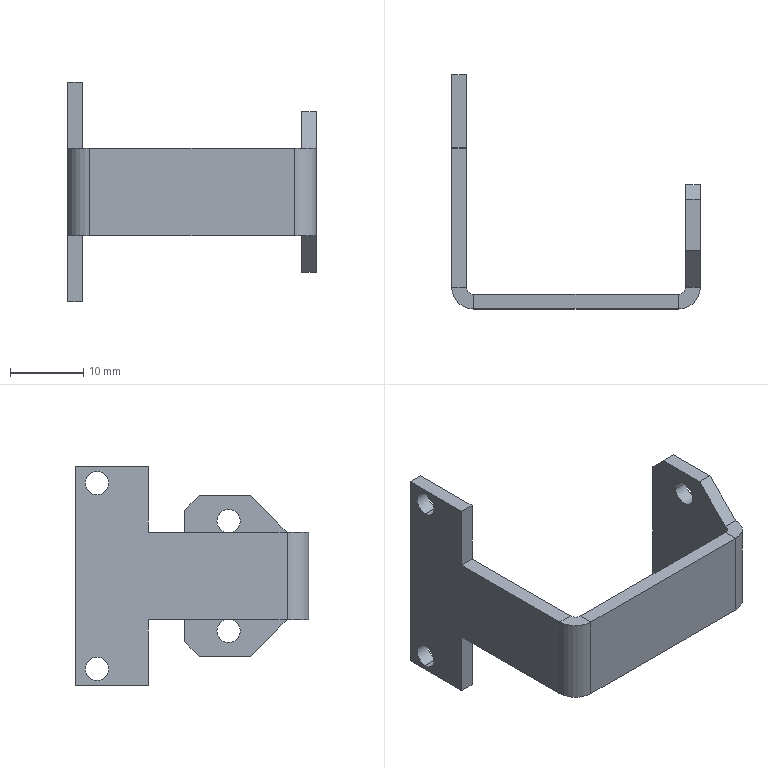Part | SolidWorks | features ICE 5, Chamfer 1, FlatPattern 1, SMBaseFlange 1, SheetMetal 1 | 1 solid | 38 faces | box 34 x 32 x 30 mm | volume 2372 mm3 | plane 26 | cylinder 12 | commonest cylinder face diameters 3.2 x8 2 x2 6 x2
STEP:
#1=CARTESIAN_POINT('',(-30.,12.,26.1));
#2=VERTEX_POINT('',#1);
#3=CARTESIAN_POINT('',(-30.,12.,29.3));
#4=VERTEX_POINT('',#3);
#5=CARTESIAN_POINT('',(-30.,12.,27.7));
#6=DIRECTION('',(-1.,0.,0.));
#7=DIRECTION('',(0.,-1.,0.));
#8=AXIS2_PLACEMENT_3D('',#5,#6,#7);
#9=CIRCLE('',#8,1.6);
#10=EDGE_CURVE('',#2,#4,#9,.T.);
#11=ORIENTED_EDGE('',*,*,#10,.F.);
#12=CARTESIAN_POINT('',(-32.,12.,26.1));
#13=VERTEX_POINT('',#12);
#14=CARTESIAN_POINT('',(-27.,12.,26.1));
#15=DIRECTION('',(-1.,0.,0.));
#16=VECTOR('',#15,1000.);
#17=LINE('',#14,#16);
#18=EDGE_CURVE('',#2,#13,#17,.T.);
#19=ORIENTED_EDGE('',*,*,#18,.T.);
#20=CARTESIAN_POINT('',(-32.,12.,29.3));
#21=VERTEX_POINT('',#20);
#22=CARTESIAN_POINT('',(-32.,12.,27.7));
#23=DIRECTION('',(-1.,0.,0.));
#24=DIRECTION('',(0.,0.,1.));
#25=AXIS2_PLACEMENT_3D('',#22,#23,#24);
#26=CIRCLE('',#25,1.6);
#27=EDGE_CURVE('',#13,#21,#26,.T.);
#28=ORIENTED_EDGE('',*,*,#27,.T.);
#29=CARTESIAN_POINT('',(-27.,12.,29.3));
#30=DIRECTION('',(-1.,0.,0.));
#31=VECTOR('',#30,1000.);
#32=LINE('',#29,#31);
#33=EDGE_CURVE('',#4,#21,#32,.T.);
#34=ORIENTED_EDGE('',*,*,#33,.F.);
#35=EDGE_LOOP('',(#11,#19,#28,#34));
#36=FACE_OUTER_BOUND('',#35,.T.);
#37=CARTESIAN_POINT('',(-27.,12.,27.7));
#38=DIRECTION('',(-1.,0.,0.));
#39=DIRECTION('',(0.,0.,1.));
#40=AXIS2_PLACEMENT_3D('',#37,#38,#39);
#41=CYLINDRICAL_SURFACE('',#40,1.6);
#42=ADVANCED_FACE('',(#36),#41,.F.);
#43=CARTESIAN_POINT('',(-30.,12.,0.7));
#44=VERTEX_POINT('',#43);
#45=CARTESIAN_POINT('',(-30.,12.,3.9));
#46=VERTEX_POINT('',#45);
#47=CARTESIAN_POINT('',(-30.,12.,2.3));
#48=DIRECTION('',(-1.,0.,0.));
#49=DIRECTION('',(0.,-1.,0.));
#50=AXIS2_PLACEMENT_3D('',#47,#48,#49);
#51=CIRCLE('',#50,1.6);
#52=EDGE_CURVE('',#44,#46,#51,.T.);
#53=ORIENTED_EDGE('',*,*,#52,.F.);
#54=CARTESIAN_POINT('',(-32.,12.,0.7));
#55=VERTEX_POINT('',#54);
#56=CARTESIAN_POINT('',(-27.,12.,0.7));
#57=DIRECTION('',(-1.,0.,0.));
#58=VECTOR('',#57,1000.);
#59=LINE('',#56,#58);
#60=EDGE_CURVE('',#44,#55,#59,.T.);
#61=ORIENTED_EDGE('',*,*,#60,.T.);
#62=CARTESIAN_POINT('',(-32.,12.,3.9));
#63=VERTEX_POINT('',#62);
#64=CARTESIAN_POINT('',(-32.,12.,2.3));
#65=DIRECTION('',(-1.,0.,0.));
#66=DIRECTION('',(0.,0.,1.));
#67=AXIS2_PLACEMENT_3D('',#64,#65,#66);
#68=CIRCLE('',#67,1.6);
#69=EDGE_CURVE('',#55,#63,#68,.T.);
#70=ORIENTED_EDGE('',*,*,#69,.T.);
#71=CARTESIAN_POINT('',(-27.,12.,3.9));
#72=DIRECTION('',(-1.,0.,0.));
#73=VECTOR('',#72,1000.);
#74=LINE('',#71,#73);
#75=EDGE_CURVE('',#46,#63,#74,.T.);
#76=ORIENTED_EDGE('',*,*,#75,.F.);
#77=EDGE_LOOP('',(#53,#61,#70,#76));
#78=FACE_OUTER_BOUND('',#77,.T.);
#79=CARTESIAN_POINT('',(-27.,12.,2.3));
#80=DIRECTION('',(-1.,0.,0.));
#81=DIRECTION('',(0.,0.,1.));
#82=AXIS2_PLACEMENT_3D('',#79,#80,#81);
#83=CYLINDRICAL_SURFACE('',#82,1.6);
#84=ADVANCED_FACE('',(#78),#83,.F.);
#85=CARTESIAN_POINT('',(0.,-7.6,7.5));
#86=VERTEX_POINT('',#85);
#87=CARTESIAN_POINT('',(0.,-4.4,7.5));
#88=VERTEX_POINT('',#87);
#89=CARTESIAN_POINT('',(0.,-6.,7.5));
#90=DIRECTION('',(1.,0.,0.));
#91=DIRECTION('',(0.,1.,0.));
#92=AXIS2_PLACEMENT_3D('',#89,#90,#91);
#93=CIRCLE('',#92,1.6);
#94=EDGE_CURVE('',#86,#88,#93,.T.);
#95=ORIENTED_EDGE('',*,*,#94,.F.);
#96=CARTESIAN_POINT('',(2.,-7.6,7.5));
#97=VERTEX_POINT('',#96);
#98=CARTESIAN_POINT('',(-8.,-7.6,7.5));
#99=DIRECTION('',(1.,0.,0.));
#100=VECTOR('',#99,1000.);
#101=LINE('',#98,#100);
#102=EDGE_CURVE('',#86,#97,#101,.T.);
#103=ORIENTED_EDGE('',*,*,#102,.T.);
#104=CARTESIAN_POINT('',(2.,-4.4,7.5));
#105=VERTEX_POINT('',#104);
#106=CARTESIAN_POINT('',(2.,-6.,7.5));
#107=DIRECTION('',(1.,0.,0.));
#108=DIRECTION('',(0.,1.,0.));
#109=AXIS2_PLACEMENT_3D('',#106,#107,#108);
#110=CIRCLE('',#109,1.6);
#111=EDGE_CURVE('',#97,#105,#110,.T.);
#112=ORIENTED_EDGE('',*,*,#111,.T.);
#113=CARTESIAN_POINT('',(-8.,-4.4,7.5));
#114=DIRECTION('',(1.,0.,0.));
#115=VECTOR('',#114,1000.);
#116=LINE('',#113,#115);
#117=EDGE_CURVE('',#88,#105,#116,.T.);
#118=ORIENTED_EDGE('',*,*,#117,.F.);
#119=EDGE_LOOP('',(#95,#103,#112,#118));
#120=FACE_OUTER_BOUND('',#119,.T.);
#121=CARTESIAN_POINT('',(-8.,-6.,7.5));
#122=DIRECTION('',(1.,0.,0.));
#123=DIRECTION('',(0.,1.,0.));
#124=AXIS2_PLACEMENT_3D('',#121,#122,#123);
#125=CYLINDRICAL_SURFACE('',#124,1.6);
#126=ADVANCED_FACE('',(#120),#125,.F.);
#127=CARTESIAN_POINT('',(0.,-7.6,22.5));
#128=VERTEX_POINT('',#127);
#129=CARTESIAN_POINT('',(0.,-4.4,22.5));
#130=VERTEX_POINT('',#129);
#131=CARTESIAN_POINT('',(0.,-6.,22.5));
#132=DIRECTION('',(1.,0.,0.));
#133=DIRECTION('',(0.,1.,0.));
#134=AXIS2_PLACEMENT_3D('',#131,#132,#133);
#135=CIRCLE('',#134,1.6);
#136=EDGE_CURVE('',#128,#130,#135,.T.);
#137=ORIENTED_EDGE('',*,*,#136,.F.);
#138=CARTESIAN_POINT('',(2.,-7.6,22.5));
#139=VERTEX_POINT('',#138);
#140=CARTESIAN_POINT('',(-8.,-7.6,22.5));
#141=DIRECTION('',(1.,0.,0.));
#142=VECTOR('',#141,1000.);
#143=LINE('',#140,#142);
#144=EDGE_CURVE('',#128,#139,#143,.T.);
#145=ORIENTED_EDGE('',*,*,#144,.T.);
#146=CARTESIAN_POINT('',(2.,-4.4,22.5));
#147=VERTEX_POINT('',#146);
#148=CARTESIAN_POINT('',(2.,-6.,22.5));
#149=DIRECTION('',(1.,0.,0.));
#150=DIRECTION('',(0.,1.,0.));
#151=AXIS2_PLACEMENT_3D('',#148,#149,#150);
#152=CIRCLE('',#151,1.6);
#153=EDGE_CURVE('',#139,#147,#152,.T.);
#154=ORIENTED_EDGE('',*,*,#153,.T.);
#155=CARTESIAN_POINT('',(-8.,-4.4,22.5));
#156=DIRECTION('',(1.,0.,0.));
#157=VECTOR('',#156,1000.);
#158=LINE('',#155,#157);
#159=EDGE_CURVE('',#130,#147,#158,.T.);
#160=ORIENTED_EDGE('',*,*,#159,.F.);
#161=EDGE_LOOP('',(#137,#145,#154,#160));
#162=FACE_OUTER_BOUND('',#161,.T.);
#163=CARTESIAN_POINT('',(-8.,-6.,22.5));
#164=DIRECTION('',(1.,0.,0.));
#165=DIRECTION('',(0.,1.,0.));
#166=AXIS2_PLACEMENT_3D('',#163,#164,#165);
#167=CYLINDRICAL_SURFACE('',#166,1.6);
#168=ADVANCED_FACE('',(#162),#167,.F.);
#169=CARTESIAN_POINT('',(2.,-6.,7.5));
#170=DIRECTION('',(1.,0.,0.));
#171=DIRECTION('',(0.,1.,0.));
#172=AXIS2_PLACEMENT_3D('',#169,#170,#171);
#173=CIRCLE('',#172,1.6);
#174=EDGE_CURVE('',#105,#97,#173,.T.);
#175=ORIENTED_EDGE('',*,*,#174,.F.);
#176=ORIENTED_EDGE('',*,*,#111,.F.);
#177=EDGE_LOOP('',(#175,#176));
#178=FACE_BOUND('',#177,.T.);
#179=CARTESIAN_POINT('',(2.,-6.,22.5));
#180=DIRECTION('',(1.,0.,0.));
#181=DIRECTION('',(0.,1.,0.));
#182=AXIS2_PLACEMENT_3D('',#179,#180,#181);
#183=CIRCLE('',#182,1.6);
#184=EDGE_CURVE('',#147,#139,#183,.T.);
#185=ORIENTED_EDGE('',*,*,#184,.F.);
#186=ORIENTED_EDGE('',*,*,#153,.F.);
#187=EDGE_LOOP('',(#185,#186));
#188=FACE_BOUND('',#187,.T.);
#189=CARTESIAN_POINT('',(2.,0.,24.));
#190=VERTEX_POINT('',#189);
#191=CARTESIAN_POINT('',(2.,0.,6.));
#192=VERTEX_POINT('',#191);
#193=CARTESIAN_POINT('',(2.,0.,30.));
#194=DIRECTION('',(0.,0.,-1.));
#195=VECTOR('',#194,1000.);
#196=LINE('',#193,#195);
#197=EDGE_CURVE('',#190,#192,#196,.T.);
#198=ORIENTED_EDGE('',*,*,#197,.F.);
#199=CARTESIAN_POINT('',(2.,-2.,26.));
#200=VERTEX_POINT('',#199);
#201=CARTESIAN_POINT('',(2.,-3.,27.));
#202=DIRECTION('',(0.,-0.7071,0.7071));
#203=VECTOR('',#202,1000.);
#204=LINE('',#201,#203);
#205=EDGE_CURVE('',#190,#200,#204,.T.);
#206=ORIENTED_EDGE('',*,*,#205,.T.);
#207=CARTESIAN_POINT('',(2.,-9.,26.));
#208=VERTEX_POINT('',#207);
#209=CARTESIAN_POINT('',(2.,0.,26.));
#210=DIRECTION('',(0.,1.,0.));
#211=VECTOR('',#210,1000.);
#212=LINE('',#209,#211);
#213=EDGE_CURVE('',#208,#200,#212,.T.);
#214=ORIENTED_EDGE('',*,*,#213,.F.);
#215=CARTESIAN_POINT('',(2.,-14.,21.));
#216=VERTEX_POINT('',#215);
#217=CARTESIAN_POINT('',(2.,-2.5,32.5));
#218=DIRECTION('',(0.,0.7071,0.7071));
#219=VECTOR('',#218,1000.);
#220=LINE('',#217,#219);
#221=EDGE_CURVE('',#216,#208,#220,.T.);
#222=ORIENTED_EDGE('',*,*,#221,.F.);
#223=CARTESIAN_POINT('',(2.,-14.,9.));
#224=VERTEX_POINT('',#223);
#225=CARTESIAN_POINT('',(2.,-14.,30.));
#226=DIRECTION('',(0.,0.,-1.));
#227=VECTOR('',#226,1000.);
#228=LINE('',#225,#227);
#229=EDGE_CURVE('',#216,#224,#228,.T.);
#230=ORIENTED_EDGE('',*,*,#229,.T.);
#231=CARTESIAN_POINT('',(2.,-9.,4.));
#232=VERTEX_POINT('',#231);
#233=CARTESIAN_POINT('',(2.,-17.5,12.5));
#234=DIRECTION('',(0.,-0.7071,0.7071));
#235=VECTOR('',#234,1000.);
#236=LINE('',#233,#235);
#237=EDGE_CURVE('',#232,#224,#236,.T.);
#238=ORIENTED_EDGE('',*,*,#237,.F.);
#239=CARTESIAN_POINT('',(2.,-2.,4.));
#240=VERTEX_POINT('',#239);
#241=CARTESIAN_POINT('',(2.,0.,4.));
#242=DIRECTION('',(0.,-1.,0.));
#243=VECTOR('',#242,1000.);
#244=LINE('',#241,#243);
#245=EDGE_CURVE('',#240,#232,#244,.T.);
#246=ORIENTED_EDGE('',*,*,#245,.F.);
#247=CARTESIAN_POINT('',(2.,12.,18.));
#248=DIRECTION('',(0.,0.7071,0.7071));
#249=VECTOR('',#248,1000.);
#250=LINE('',#247,#249);
#251=EDGE_CURVE('',#240,#192,#250,.T.);
#252=ORIENTED_EDGE('',*,*,#251,.T.);
#253=EDGE_LOOP('',(#198,#206,#214,#222,#230,#238,#246,#252));
#254=FACE_OUTER_BOUND('',#253,.T.);
#255=CARTESIAN_POINT('',(2.,0.,30.));
#256=DIRECTION('',(1.,0.,0.));
#257=DIRECTION('',(0.,1.,0.));
#258=AXIS2_PLACEMENT_3D('',#255,#256,#257);
#259=PLANE('',#258);
#260=ADVANCED_FACE('',(#178,#188,#254),#259,.T.);
#261=CARTESIAN_POINT('',(0.,-6.,7.5));
#262=DIRECTION('',(1.,0.,0.));
#263=DIRECTION('',(0.,1.,0.));
#264=AXIS2_PLACEMENT_3D('',#261,#262,#263);
#265=CIRCLE('',#264,1.6);
#266=EDGE_CURVE('',#88,#86,#265,.T.);
#267=ORIENTED_EDGE('',*,*,#266,.T.);
#268=ORIENTED_EDGE('',*,*,#94,.T.);
#269=EDGE_LOOP('',(#267,#268));
#270=FACE_BOUND('',#269,.T.);
#271=CARTESIAN_POINT('',(0.,-6.,22.5));
#272=DIRECTION('',(1.,0.,0.));
#273=DIRECTION('',(0.,1.,0.));
#274=AXIS2_PLACEMENT_3D('',#271,#272,#273);
#275=CIRCLE('',#274,1.6);
#276=EDGE_CURVE('',#130,#128,#275,.T.);
#277=ORIENTED_EDGE('',*,*,#276,.T.);
#278=ORIENTED_EDGE('',*,*,#136,.T.);
#279=EDGE_LOOP('',(#277,#278));
#280=FACE_BOUND('',#279,.T.);
#281=CARTESIAN_POINT('',(0.,-9.,26.));
#282=VERTEX_POINT('',#281);
#283=CARTESIAN_POINT('',(0.,-2.,26.));
#284=VERTEX_POINT('',#283);
#285=CARTESIAN_POINT('',(0.,0.,26.));
#286=DIRECTION('',(0.,1.,0.));
#287=VECTOR('',#286,1000.);
#288=LINE('',#285,#287);
#289=EDGE_CURVE('',#282,#284,#288,.T.);
#290=ORIENTED_EDGE('',*,*,#289,.T.);
#291=CARTESIAN_POINT('',(0.,0.,24.));
#292=VERTEX_POINT('',#291);
#293=CARTESIAN_POINT('',(0.,0.,24.));
#294=DIRECTION('',(0.,0.7071,-0.7071));
#295=VECTOR('',#294,1000.);
#296=LINE('',#293,#295);
#297=EDGE_CURVE('',#284,#292,#296,.T.);
#298=ORIENTED_EDGE('',*,*,#297,.T.);
#299=CARTESIAN_POINT('',(0.,0.,6.));
#300=VERTEX_POINT('',#299);
#301=CARTESIAN_POINT('',(0.,0.,30.));
#302=DIRECTION('',(0.,0.,-1.));
#303=VECTOR('',#302,1000.);
#304=LINE('',#301,#303);
#305=EDGE_CURVE('',#292,#300,#304,.T.);
#306=ORIENTED_EDGE('',*,*,#305,.T.);
#307=CARTESIAN_POINT('',(0.,-2.,4.));
#308=VERTEX_POINT('',#307);
#309=CARTESIAN_POINT('',(0.,-2.,4.));
#310=DIRECTION('',(0.,-0.7071,-0.7071));
#311=VECTOR('',#310,1000.);
#312=LINE('',#309,#311);
#313=EDGE_CURVE('',#300,#308,#312,.T.);
#314=ORIENTED_EDGE('',*,*,#313,.T.);
#315=CARTESIAN_POINT('',(0.,-9.,4.));
#316=VERTEX_POINT('',#315);
#317=CARTESIAN_POINT('',(0.,0.,4.));
#318=DIRECTION('',(0.,-1.,0.));
#319=VECTOR('',#318,1000.);
#320=LINE('',#317,#319);
#321=EDGE_CURVE('',#308,#316,#320,.T.);
#322=ORIENTED_EDGE('',*,*,#321,.T.);
#323=CARTESIAN_POINT('',(0.,-14.,9.));
#324=VERTEX_POINT('',#323);
#325=CARTESIAN_POINT('',(0.,-17.5,12.5));
#326=DIRECTION('',(0.,-0.7071,0.7071));
#327=VECTOR('',#326,1000.);
#328=LINE('',#325,#327);
#329=EDGE_CURVE('',#316,#324,#328,.T.);
#330=ORIENTED_EDGE('',*,*,#329,.T.);
#331=CARTESIAN_POINT('',(0.,-14.,21.));
#332=VERTEX_POINT('',#331);
#333=CARTESIAN_POINT('',(0.,-14.,30.));
#334=DIRECTION('',(0.,0.,-1.));
#335=VECTOR('',#334,1000.);
#336=LINE('',#333,#335);
#337=EDGE_CURVE('',#332,#324,#336,.T.);
#338=ORIENTED_EDGE('',*,*,#337,.F.);
#339=CARTESIAN_POINT('',(0.,-2.5,32.5));
#340=DIRECTION('',(0.,0.7071,0.7071));
#341=VECTOR('',#340,1000.);
#342=LINE('',#339,#341);
#343=EDGE_CURVE('',#332,#282,#342,.T.);
#344=ORIENTED_EDGE('',*,*,#343,.T.);
#345=EDGE_LOOP('',(#290,#298,#306,#314,#322,#330,#338,#344));
#346=FACE_OUTER_BOUND('',#345,.T.);
#347=CARTESIAN_POINT('',(0.,0.,30.));
#348=DIRECTION('',(1.,0.,0.));
#349=DIRECTION('',(0.,1.,0.));
#350=AXIS2_PLACEMENT_3D('',#347,#348,#349);
#351=PLANE('',#350);
#352=ADVANCED_FACE('',(#270,#280,#346),#351,.F.);
#353=ORIENTED_EDGE('',*,*,#213,.T.);
#354=CARTESIAN_POINT('',(0.,-2.,26.));
#355=DIRECTION('',(-1.,0.,0.));
#356=VECTOR('',#355,1000.);
#357=LINE('',#354,#356);
#358=EDGE_CURVE('',#200,#284,#357,.T.);
#359=ORIENTED_EDGE('',*,*,#358,.T.);
#360=ORIENTED_EDGE('',*,*,#289,.F.);
#361=CARTESIAN_POINT('',(0.,-9.,26.));
#362=DIRECTION('',(1.,0.,0.));
#363=VECTOR('',#362,1000.);
#364=LINE('',#361,#363);
#365=EDGE_CURVE('',#282,#208,#364,.T.);
#366=ORIENTED_EDGE('',*,*,#365,.T.);
#367=EDGE_LOOP('',(#353,#359,#360,#366));
#368=FACE_OUTER_BOUND('',#367,.T.);
#369=CARTESIAN_POINT('',(-8.,0.,26.));
#370=DIRECTION('',(0.,0.,-1.));
#371=DIRECTION('',(0.,1.,0.));
#372=AXIS2_PLACEMENT_3D('',#369,#370,#371);
#373=PLANE('',#372);
#374=ADVANCED_FACE('',(#368),#373,.F.);
#375=ORIENTED_EDGE('',*,*,#321,.F.);
#376=CARTESIAN_POINT('',(2.,-2.,4.));
#377=DIRECTION('',(1.,0.,0.));
#378=VECTOR('',#377,1000.);
#379=LINE('',#376,#378);
#380=EDGE_CURVE('',#308,#240,#379,.T.);
#381=ORIENTED_EDGE('',*,*,#380,.T.);
#382=ORIENTED_EDGE('',*,*,#245,.T.);
#383=CARTESIAN_POINT('',(0.,-9.,4.));
#384=DIRECTION('',(1.,0.,0.));
#385=VECTOR('',#384,1000.);
#386=LINE('',#383,#385);
#387=EDGE_CURVE('',#316,#232,#386,.T.);
#388=ORIENTED_EDGE('',*,*,#387,.F.);
#389=EDGE_LOOP('',(#375,#381,#382,#388));
#390=FACE_OUTER_BOUND('',#389,.T.);
#391=CARTESIAN_POINT('',(-8.,0.,4.));
#392=DIRECTION('',(0.,0.,1.));
#393=DIRECTION('',(1.,0.,0.));
#394=AXIS2_PLACEMENT_3D('',#391,#392,#393);
#395=PLANE('',#394);
#396=ADVANCED_FACE('',(#390),#395,.F.);
#397=CARTESIAN_POINT('',(-30.,12.,27.7));
#398=DIRECTION('',(-1.,0.,0.));
#399=DIRECTION('',(0.,-1.,0.));
#400=AXIS2_PLACEMENT_3D('',#397,#398,#399);
#401=CIRCLE('',#400,1.6);
#402=EDGE_CURVE('',#4,#2,#401,.T.);
#403=ORIENTED_EDGE('',*,*,#402,.T.);
#404=ORIENTED_EDGE('',*,*,#10,.T.);
#405=EDGE_LOOP('',(#403,#404));
#406=FACE_BOUND('',#405,.T.);
#407=CARTESIAN_POINT('',(-30.,12.,2.3));
#408=DIRECTION('',(-1.,0.,0.));
#409=DIRECTION('',(0.,-1.,0.));
#410=AXIS2_PLACEMENT_3D('',#407,#408,#409);
#411=CIRCLE('',#410,1.6);
#412=EDGE_CURVE('',#46,#44,#411,.T.);
#413=ORIENTED_EDGE('',*,*,#412,.T.);
#414=ORIENTED_EDGE('',*,*,#52,.T.);
#415=EDGE_LOOP('',(#413,#414));
#416=FACE_BOUND('',#415,.T.);
#417=CARTESIAN_POINT('',(-30.,5.,9.));
#418=VERTEX_POINT('',#417);
#419=CARTESIAN_POINT('',(-30.,5.,0.));
#420=VERTEX_POINT('',#419);
#421=CARTESIAN_POINT('',(-30.,5.,30.));
#422=DIRECTION('',(0.,0.,-1.));
#423=VECTOR('',#422,1000.);
#424=LINE('',#421,#423);
#425=EDGE_CURVE('',#418,#420,#424,.T.);
#426=ORIENTED_EDGE('',*,*,#425,.T.);
#427=CARTESIAN_POINT('',(-30.,15.,0.));
#428=VERTEX_POINT('',#427);
#429=CARTESIAN_POINT('',(-30.,-15.,0.));
#430=DIRECTION('',(0.,1.,0.));
#431=VECTOR('',#430,1000.);
#432=LINE('',#429,#431);
#433=EDGE_CURVE('',#420,#428,#432,.T.);
#434=ORIENTED_EDGE('',*,*,#433,.T.);
#435=CARTESIAN_POINT('',(-30.,15.,30.));
#436=VERTEX_POINT('',#435);
#437=CARTESIAN_POINT('',(-30.,15.,30.));
#438=DIRECTION('',(0.,0.,-1.));
#439=VECTOR('',#438,1000.);
#440=LINE('',#437,#439);
#441=EDGE_CURVE('',#436,#428,#440,.T.);
#442=ORIENTED_EDGE('',*,*,#441,.F.);
#443=CARTESIAN_POINT('',(-30.,5.,30.));
#444=VERTEX_POINT('',#443);
#445=CARTESIAN_POINT('',(-30.,-15.,30.));
#446=DIRECTION('',(0.,1.,0.));
#447=VECTOR('',#446,1000.);
#448=LINE('',#445,#447);
#449=EDGE_CURVE('',#444,#436,#448,.T.);
#450=ORIENTED_EDGE('',*,*,#449,.F.);
#451=CARTESIAN_POINT('',(-30.,5.,21.));
#452=VERTEX_POINT('',#451);
#453=CARTESIAN_POINT('',(-30.,5.,30.));
#454=DIRECTION('',(0.,0.,-1.));
#455=VECTOR('',#454,1000.);
#456=LINE('',#453,#455);
#457=EDGE_CURVE('',#444,#452,#456,.T.);
#458=ORIENTED_EDGE('',*,*,#457,.T.);
#459=CARTESIAN_POINT('',(-30.,-14.,21.));
#460=VERTEX_POINT('',#459);
#461=CARTESIAN_POINT('',(-30.,-15.,21.));
#462=DIRECTION('',(0.,-1.,0.));
#463=VECTOR('',#462,1000.);
#464=LINE('',#461,#463);
#465=EDGE_CURVE('',#452,#460,#464,.T.);
#466=ORIENTED_EDGE('',*,*,#465,.T.);
#467=CARTESIAN_POINT('',(-30.,-14.,9.));
#468=VERTEX_POINT('',#467);
#469=CARTESIAN_POINT('',(-30.,-14.,30.));
#470=DIRECTION('',(0.,0.,-1.));
#471=VECTOR('',#470,1000.);
#472=LINE('',#469,#471);
#473=EDGE_CURVE('',#460,#468,#472,.T.);
#474=ORIENTED_EDGE('',*,*,#473,.T.);
#475=CARTESIAN_POINT('',(-30.,-15.,9.));
#476=DIRECTION('',(0.,1.,0.));
#477=VECTOR('',#476,1000.);
#478=LINE('',#475,#477);
#479=EDGE_CURVE('',#468,#418,#478,.T.);
#480=ORIENTED_EDGE('',*,*,#479,.T.);
#481=EDGE_LOOP('',(#426,#434,#442,#450,#458,#466,#474,#480));
#482=FACE_OUTER_BOUND('',#481,.T.);
#483=CARTESIAN_POINT('',(-30.,-15.,30.));
#484=DIRECTION('',(-1.,0.,0.));
#485=DIRECTION('',(0.,-1.,0.));
#486=AXIS2_PLACEMENT_3D('',#483,#484,#485);
#487=PLANE('',#486);
#488=ADVANCED_FACE('',(#406,#416,#482),#487,.F.);
#489=CARTESIAN_POINT('',(-32.,12.,27.7));
#490=DIRECTION('',(-1.,0.,0.));
#491=DIRECTION('',(0.,0.,1.));
#492=AXIS2_PLACEMENT_3D('',#489,#490,#491);
#493=CIRCLE('',#492,1.6);
#494=EDGE_CURVE('',#21,#13,#493,.T.);
#495=ORIENTED_EDGE('',*,*,#494,.F.);
#496=ORIENTED_EDGE('',*,*,#27,.F.);
#497=EDGE_LOOP('',(#495,#496));
#498=FACE_BOUND('',#497,.T.);
#499=CARTESIAN_POINT('',(-32.,12.,2.3));
#500=DIRECTION('',(-1.,0.,0.));
#501=DIRECTION('',(0.,0.,1.));
#502=AXIS2_PLACEMENT_3D('',#499,#500,#501);
#503=CIRCLE('',#502,1.6);
#504=EDGE_CURVE('',#63,#55,#503,.T.);
#505=ORIENTED_EDGE('',*,*,#504,.F.);
#506=ORIENTED_EDGE('',*,*,#69,.F.);
#507=EDGE_LOOP('',(#505,#506));
#508=FACE_BOUND('',#507,.T.);
#509=CARTESIAN_POINT('',(-32.,5.,0.));
#510=VERTEX_POINT('',#509);
#511=CARTESIAN_POINT('',(-32.,15.,0.));
#512=VERTEX_POINT('',#511);
#513=CARTESIAN_POINT('',(-32.,-15.,0.));
#514=DIRECTION('',(0.,1.,0.));
#515=VECTOR('',#514,1000.);
#516=LINE('',#513,#515);
#517=EDGE_CURVE('',#510,#512,#516,.T.);
#518=ORIENTED_EDGE('',*,*,#517,.F.);
#519=CARTESIAN_POINT('',(-32.,5.,9.));
#520=VERTEX_POINT('',#519);
#521=CARTESIAN_POINT('',(-32.,5.,30.));
#522=DIRECTION('',(0.,0.,-1.));
#523=VECTOR('',#522,1000.);
#524=LINE('',#521,#523);
#525=EDGE_CURVE('',#520,#510,#524,.T.);
#526=ORIENTED_EDGE('',*,*,#525,.F.);
#527=CARTESIAN_POINT('',(-32.,-14.,9.));
#528=VERTEX_POINT('',#527);
#529=CARTESIAN_POINT('',(-32.,-15.,9.));
#530=DIRECTION('',(0.,1.,0.));
#531=VECTOR('',#530,1000.);
#532=LINE('',#529,#531);
#533=EDGE_CURVE('',#528,#520,#532,.T.);
#534=ORIENTED_EDGE('',*,*,#533,.F.);
#535=CARTESIAN_POINT('',(-32.,-14.,21.));
#536=VERTEX_POINT('',#535);
#537=CARTESIAN_POINT('',(-32.,-14.,30.));
#538=DIRECTION('',(0.,0.,-1.));
#539=VECTOR('',#538,1000.);
#540=LINE('',#537,#539);
#541=EDGE_CURVE('',#536,#528,#540,.T.);
#542=ORIENTED_EDGE('',*,*,#541,.F.);
#543=CARTESIAN_POINT('',(-32.,5.,21.));
#544=VERTEX_POINT('',#543);
#545=CARTESIAN_POINT('',(-32.,-15.,21.));
#546=DIRECTION('',(0.,-1.,0.));
#547=VECTOR('',#546,1000.);
#548=LINE('',#545,#547);
#549=EDGE_CURVE('',#544,#536,#548,.T.);
#550=ORIENTED_EDGE('',*,*,#549,.F.);
#551=CARTESIAN_POINT('',(-32.,5.,30.));
#552=VERTEX_POINT('',#551);
#553=CARTESIAN_POINT('',(-32.,5.,30.));
#554=DIRECTION('',(0.,0.,-1.));
#555=VECTOR('',#554,1000.);
#556=LINE('',#553,#555);
#557=EDGE_CURVE('',#552,#544,#556,.T.);
#558=ORIENTED_EDGE('',*,*,#557,.F.);
#559=CARTESIAN_POINT('',(-32.,15.,30.));
#560=VERTEX_POINT('',#559);
#561=CARTESIAN_POINT('',(-32.,-15.,30.));
#562=DIRECTION('',(0.,1.,0.));
#563=VECTOR('',#562,1000.);
#564=LINE('',#561,#563);
#565=EDGE_CURVE('',#552,#560,#564,.T.);
#566=ORIENTED_EDGE('',*,*,#565,.T.);
#567=CARTESIAN_POINT('',(-32.,15.,30.));
#568=DIRECTION('',(0.,0.,-1.));
#569=VECTOR('',#568,1000.);
#570=LINE('',#567,#569);
#571=EDGE_CURVE('',#560,#512,#570,.T.);
#572=ORIENTED_EDGE('',*,*,#571,.T.);
#573=EDGE_LOOP('',(#518,#526,#534,#542,#550,#558,#566,#572));
#574=FACE_OUTER_BOUND('',#573,.T.);
#575=CARTESIAN_POINT('',(-32.,-15.,30.));
#576=DIRECTION('',(-1.,0.,0.));
#577=DIRECTION('',(0.,-1.,0.));
#578=AXIS2_PLACEMENT_3D('',#575,#576,#577);
#579=PLANE('',#578);
#580=ADVANCED_FACE('',(#498,#508,#574),#579,.T.);
#581=ORIENTED_EDGE('',*,*,#541,.T.);
#582=CARTESIAN_POINT('',(-29.,-17.,9.));
#583=VERTEX_POINT('',#582);
#584=CARTESIAN_POINT('',(-29.,-14.,9.));
#585=DIRECTION('',(0.,0.,-1.));
#586=DIRECTION('',(0.,-1.,0.));
#587=AXIS2_PLACEMENT_3D('',#584,#585,#586);
#588=CIRCLE('',#587,3.);
#589=EDGE_CURVE('',#583,#528,#588,.T.);
#590=ORIENTED_EDGE('',*,*,#589,.F.);
#591=CARTESIAN_POINT('',(-29.,-17.,21.));
#592=VERTEX_POINT('',#591);
#593=CARTESIAN_POINT('',(-29.,-17.,30.));
#594=DIRECTION('',(0.,0.,-1.));
#595=VECTOR('',#594,1000.);
#596=LINE('',#593,#595);
#597=EDGE_CURVE('',#592,#583,#596,.T.);
#598=ORIENTED_EDGE('',*,*,#597,.F.);
#599=CARTESIAN_POINT('',(-29.,-14.,21.));
#600=DIRECTION('',(0.,0.,1.));
#601=DIRECTION('',(0.,1.,0.));
#602=AXIS2_PLACEMENT_3D('',#599,#600,#601);
#603=CIRCLE('',#602,3.);
#604=EDGE_CURVE('',#536,#592,#603,.T.);
#605=ORIENTED_EDGE('',*,*,#604,.F.);
#606=EDGE_LOOP('',(#581,#590,#598,#605));
#607=FACE_OUTER_BOUND('',#606,.T.);
#608=CARTESIAN_POINT('',(-29.,-14.,30.));
#609=DIRECTION('',(0.,0.,-1.));
#610=DIRECTION('',(-1.,0.,0.));
#611=AXIS2_PLACEMENT_3D('',#608,#609,#610);
#612=CYLINDRICAL_SURFACE('',#611,3.);
#613=ADVANCED_FACE('',(#607),#612,.T.);
#614=ORIENTED_EDGE('',*,*,#597,.T.);
#615=CARTESIAN_POINT('',(-1.,-17.,9.));
#616=VERTEX_POINT('',#615);
#617=CARTESIAN_POINT('',(0.,-17.,9.));
#618=DIRECTION('',(-1.,0.,0.));
#619=VECTOR('',#618,1000.);
#620=LINE('',#617,#619);
#621=EDGE_CURVE('',#616,#583,#620,.T.);
#622=ORIENTED_EDGE('',*,*,#621,.F.);
#623=CARTESIAN_POINT('',(-1.,-17.,21.));
#624=VERTEX_POINT('',#623);
#625=CARTESIAN_POINT('',(-1.,-17.,30.));
#626=DIRECTION('',(0.,0.,-1.));
#627=VECTOR('',#626,1000.);
#628=LINE('',#625,#627);
#629=EDGE_CURVE('',#624,#616,#628,.T.);
#630=ORIENTED_EDGE('',*,*,#629,.F.);
#631=CARTESIAN_POINT('',(0.,-17.,21.));
#632=DIRECTION('',(1.,0.,0.));
#633=VECTOR('',#632,1000.);
#634=LINE('',#631,#633);
#635=EDGE_CURVE('',#592,#624,#634,.T.);
#636=ORIENTED_EDGE('',*,*,#635,.F.);
#637=EDGE_LOOP('',(#614,#622,#630,#636));
#638=FACE_OUTER_BOUND('',#637,.T.);
#639=CARTESIAN_POINT('',(0.,-17.,30.));
#640=DIRECTION('',(0.,-1.,0.));
#641=DIRECTION('',(1.,0.,0.));
#642=AXIS2_PLACEMENT_3D('',#639,#640,#641);
#643=PLANE('',#642);
#644=ADVANCED_FACE('',(#638),#643,.T.);
#645=ORIENTED_EDGE('',*,*,#629,.T.);
#646=CARTESIAN_POINT('',(-1.,-14.,9.));
#647=DIRECTION('',(0.,0.,-1.));
#648=DIRECTION('',(0.,-1.,0.));
#649=AXIS2_PLACEMENT_3D('',#646,#647,#648);
#650=CIRCLE('',#649,3.);
#651=EDGE_CURVE('',#224,#616,#650,.T.);
#652=ORIENTED_EDGE('',*,*,#651,.F.);
#653=ORIENTED_EDGE('',*,*,#229,.F.);
#654=CARTESIAN_POINT('',(-1.,-14.,21.));
#655=DIRECTION('',(0.,0.,1.));
#656=DIRECTION('',(-1.,0.,0.));
#657=AXIS2_PLACEMENT_3D('',#654,#655,#656);
#658=CIRCLE('',#657,3.);
#659=EDGE_CURVE('',#624,#216,#658,.T.);
#660=ORIENTED_EDGE('',*,*,#659,.F.);
#661=EDGE_LOOP('',(#645,#652,#653,#660));
#662=FACE_OUTER_BOUND('',#661,.T.);
#663=CARTESIAN_POINT('',(-1.,-14.,30.));
#664=DIRECTION('',(0.,0.,-1.));
#665=DIRECTION('',(-1.,0.,0.));
#666=AXIS2_PLACEMENT_3D('',#663,#664,#665);
#667=CYLINDRICAL_SURFACE('',#666,3.);
#668=ADVANCED_FACE('',(#662),#667,.T.);
#669=CARTESIAN_POINT('',(-1.,-15.,9.));
#670=VERTEX_POINT('',#669);
#671=CARTESIAN_POINT('',(-1.,-14.,9.));
#672=DIRECTION('',(0.,0.,-1.));
#673=DIRECTION('',(-1.,0.,0.));
#674=AXIS2_PLACEMENT_3D('',#671,#672,#673);
#675=CIRCLE('',#674,1.);
#676=EDGE_CURVE('',#324,#670,#675,.T.);
#677=ORIENTED_EDGE('',*,*,#676,.T.);
#678=CARTESIAN_POINT('',(-1.,-15.,21.));
#679=VERTEX_POINT('',#678);
#680=CARTESIAN_POINT('',(-1.,-15.,30.));
#681=DIRECTION('',(0.,0.,-1.));
#682=VECTOR('',#681,1000.);
#683=LINE('',#680,#682);
#684=EDGE_CURVE('',#679,#670,#683,.T.);
#685=ORIENTED_EDGE('',*,*,#684,.F.);
#686=CARTESIAN_POINT('',(-1.,-14.,21.));
#687=DIRECTION('',(0.,0.,1.));
#688=DIRECTION('',(0.,1.,0.));
#689=AXIS2_PLACEMENT_3D('',#686,#687,#688);
#690=CIRCLE('',#689,1.);
#691=EDGE_CURVE('',#679,#332,#690,.T.);
#692=ORIENTED_EDGE('',*,*,#691,.T.);
#693=ORIENTED_EDGE('',*,*,#337,.T.);
#694=EDGE_LOOP('',(#677,#685,#692,#693));
#695=FACE_OUTER_BOUND('',#694,.T.);
#696=CARTESIAN_POINT('',(-1.,-14.,30.));
#697=DIRECTION('',(0.,0.,-1.));
#698=DIRECTION('',(-1.,0.,0.));
#699=AXIS2_PLACEMENT_3D('',#696,#697,#698);
#700=CYLINDRICAL_SURFACE('',#699,1.);
#701=ADVANCED_FACE('',(#695),#700,.F.);
#702=CARTESIAN_POINT('',(-29.,-15.,9.));
#703=VERTEX_POINT('',#702);
#704=CARTESIAN_POINT('',(0.,-15.,9.));
#705=DIRECTION('',(-1.,0.,0.));
#706=VECTOR('',#705,1000.);
#707=LINE('',#704,#706);
#708=EDGE_CURVE('',#670,#703,#707,.T.);
#709=ORIENTED_EDGE('',*,*,#708,.T.);
#710=CARTESIAN_POINT('',(-29.,-15.,21.));
#711=VERTEX_POINT('',#710);
#712=CARTESIAN_POINT('',(-29.,-15.,30.));
#713=DIRECTION('',(0.,0.,-1.));
#714=VECTOR('',#713,1000.);
#715=LINE('',#712,#714);
#716=EDGE_CURVE('',#711,#703,#715,.T.);
#717=ORIENTED_EDGE('',*,*,#716,.F.);
#718=CARTESIAN_POINT('',(0.,-15.,21.));
#719=DIRECTION('',(1.,0.,0.));
#720=VECTOR('',#719,1000.);
#721=LINE('',#718,#720);
#722=EDGE_CURVE('',#711,#679,#721,.T.);
#723=ORIENTED_EDGE('',*,*,#722,.T.);
#724=ORIENTED_EDGE('',*,*,#684,.T.);
#725=EDGE_LOOP('',(#709,#717,#723,#724));
#726=FACE_OUTER_BOUND('',#725,.T.);
#727=CARTESIAN_POINT('',(0.,-15.,30.));
#728=DIRECTION('',(0.,-1.,0.));
#729=DIRECTION('',(1.,0.,0.));
#730=AXIS2_PLACEMENT_3D('',#727,#728,#729);
#731=PLANE('',#730);
#732=ADVANCED_FACE('',(#726),#731,.F.);
#733=CARTESIAN_POINT('',(-29.,-14.,9.));
#734=DIRECTION('',(0.,0.,-1.));
#735=DIRECTION('',(-1.,0.,0.));
#736=AXIS2_PLACEMENT_3D('',#733,#734,#735);
#737=CIRCLE('',#736,1.);
#738=EDGE_CURVE('',#703,#468,#737,.T.);
#739=ORIENTED_EDGE('',*,*,#738,.T.);
#740=ORIENTED_EDGE('',*,*,#473,.F.);
#741=CARTESIAN_POINT('',(-29.,-14.,21.));
#742=DIRECTION('',(0.,0.,1.));
#743=DIRECTION('',(-1.,0.,0.));
#744=AXIS2_PLACEMENT_3D('',#741,#742,#743);
#745=CIRCLE('',#744,1.);
#746=EDGE_CURVE('',#460,#711,#745,.T.);
#747=ORIENTED_EDGE('',*,*,#746,.T.);
#748=ORIENTED_EDGE('',*,*,#716,.T.);
#749=EDGE_LOOP('',(#739,#740,#747,#748));
#750=FACE_OUTER_BOUND('',#749,.T.);
#751=CARTESIAN_POINT('',(-29.,-14.,30.));
#752=DIRECTION('',(0.,0.,-1.));
#753=DIRECTION('',(-1.,0.,0.));
#754=AXIS2_PLACEMENT_3D('',#751,#752,#753);
#755=CYLINDRICAL_SURFACE('',#754,1.);
#756=ADVANCED_FACE('',(#750),#755,.F.);
#757=ORIENTED_EDGE('',*,*,#433,.F.);
#758=CARTESIAN_POINT('',(-30.,5.,0.));
#759=DIRECTION('',(-1.,0.,0.));
#760=VECTOR('',#759,1000.);
#761=LINE('',#758,#760);
#762=EDGE_CURVE('',#420,#510,#761,.T.);
#763=ORIENTED_EDGE('',*,*,#762,.T.);
#764=ORIENTED_EDGE('',*,*,#517,.T.);
#765=CARTESIAN_POINT('',(-32.,15.,0.));
#766=DIRECTION('',(1.,0.,0.));
#767=VECTOR('',#766,1000.);
#768=LINE('',#765,#767);
#769=EDGE_CURVE('',#512,#428,#768,.T.);
#770=ORIENTED_EDGE('',*,*,#769,.T.);
#771=EDGE_LOOP('',(#757,#763,#764,#770));
#772=FACE_OUTER_BOUND('',#771,.T.);
#773=CARTESIAN_POINT('',(-29.,-17.,0.));
#774=DIRECTION('',(0.,0.,-1.));
#775=DIRECTION('',(-1.,0.,0.));
#776=AXIS2_PLACEMENT_3D('',#773,#774,#775);
#777=PLANE('',#776);
#778=ADVANCED_FACE('',(#772),#777,.T.);
#779=ORIENTED_EDGE('',*,*,#565,.F.);
#780=CARTESIAN_POINT('',(-30.,5.,30.));
#781=DIRECTION('',(-1.,0.,0.));
#782=VECTOR('',#781,1000.);
#783=LINE('',#780,#782);
#784=EDGE_CURVE('',#444,#552,#783,.T.);
#785=ORIENTED_EDGE('',*,*,#784,.F.);
#786=ORIENTED_EDGE('',*,*,#449,.T.);
#787=CARTESIAN_POINT('',(-32.,15.,30.));
#788=DIRECTION('',(1.,0.,0.));
#789=VECTOR('',#788,1000.);
#790=LINE('',#787,#789);
#791=EDGE_CURVE('',#560,#436,#790,.T.);
#792=ORIENTED_EDGE('',*,*,#791,.F.);
#793=EDGE_LOOP('',(#779,#785,#786,#792));
#794=FACE_OUTER_BOUND('',#793,.T.);
#795=CARTESIAN_POINT('',(-29.,-14.,30.));
#796=DIRECTION('',(0.,0.,1.));
#797=DIRECTION('',(1.,0.,0.));
#798=AXIS2_PLACEMENT_3D('',#795,#796,#797);
#799=PLANE('',#798);
#800=ADVANCED_FACE('',(#794),#799,.T.);
#801=ORIENTED_EDGE('',*,*,#769,.F.);
#802=ORIENTED_EDGE('',*,*,#571,.F.);
#803=ORIENTED_EDGE('',*,*,#791,.T.);
#804=ORIENTED_EDGE('',*,*,#441,.T.);
#805=EDGE_LOOP('',(#801,#802,#803,#804));
#806=FACE_OUTER_BOUND('',#805,.T.);
#807=CARTESIAN_POINT('',(-32.,15.,30.));
#808=DIRECTION('',(0.,1.,0.));
#809=DIRECTION('',(0.,0.,1.));
#810=AXIS2_PLACEMENT_3D('',#807,#808,#809);
#811=PLANE('',#810);
#812=ADVANCED_FACE('',(#806),#811,.T.);
#813=ORIENTED_EDGE('',*,*,#305,.F.);
#814=CARTESIAN_POINT('',(2.,0.,24.));
#815=DIRECTION('',(1.,0.,0.));
#816=VECTOR('',#815,1000.);
#817=LINE('',#814,#816);
#818=EDGE_CURVE('',#292,#190,#817,.T.);
#819=ORIENTED_EDGE('',*,*,#818,.T.);
#820=ORIENTED_EDGE('',*,*,#197,.T.);
#821=CARTESIAN_POINT('',(0.,0.,6.));
#822=DIRECTION('',(-1.,0.,0.));
#823=VECTOR('',#822,1000.);
#824=LINE('',#821,#823);
#825=EDGE_CURVE('',#192,#300,#824,.T.);
#826=ORIENTED_EDGE('',*,*,#825,.T.);
#827=EDGE_LOOP('',(#813,#819,#820,#826));
#828=FACE_OUTER_BOUND('',#827,.T.);
#829=CARTESIAN_POINT('',(0.,0.,30.));
#830=DIRECTION('',(0.,1.,0.));
#831=DIRECTION('',(-1.,0.,0.));
#832=AXIS2_PLACEMENT_3D('',#829,#830,#831);
#833=PLANE('',#832);
#834=ADVANCED_FACE('',(#828),#833,.T.);
#835=ORIENTED_EDGE('',*,*,#144,.F.);
#836=ORIENTED_EDGE('',*,*,#276,.F.);
#837=ORIENTED_EDGE('',*,*,#159,.T.);
#838=ORIENTED_EDGE('',*,*,#184,.T.);
#839=EDGE_LOOP('',(#835,#836,#837,#838));
#840=FACE_OUTER_BOUND('',#839,.T.);
#841=CARTESIAN_POINT('',(-8.,-6.,22.5));
#842=DIRECTION('',(1.,0.,0.));
#843=DIRECTION('',(0.,1.,0.));
#844=AXIS2_PLACEMENT_3D('',#841,#842,#843);
#845=CYLINDRICAL_SURFACE('',#844,1.6);
#846=ADVANCED_FACE('',(#840),#845,.F.);
#847=ORIENTED_EDGE('',*,*,#102,.F.);
#848=ORIENTED_EDGE('',*,*,#266,.F.);
#849=ORIENTED_EDGE('',*,*,#117,.T.);
#850=ORIENTED_EDGE('',*,*,#174,.T.);
#851=EDGE_LOOP('',(#847,#848,#849,#850));
#852=FACE_OUTER_BOUND('',#851,.T.);
#853=CARTESIAN_POINT('',(-8.,-6.,7.5));
#854=DIRECTION('',(1.,0.,0.));
#855=DIRECTION('',(0.,1.,0.));
#856=AXIS2_PLACEMENT_3D('',#853,#854,#855);
#857=CYLINDRICAL_SURFACE('',#856,1.6);
#858=ADVANCED_FACE('',(#852),#857,.F.);
#859=ORIENTED_EDGE('',*,*,#60,.F.);
#860=ORIENTED_EDGE('',*,*,#412,.F.);
#861=ORIENTED_EDGE('',*,*,#75,.T.);
#862=ORIENTED_EDGE('',*,*,#504,.T.);
#863=EDGE_LOOP('',(#859,#860,#861,#862));
#864=FACE_OUTER_BOUND('',#863,.T.);
#865=CARTESIAN_POINT('',(-27.,12.,2.3));
#866=DIRECTION('',(-1.,0.,0.));
#867=DIRECTION('',(0.,0.,1.));
#868=AXIS2_PLACEMENT_3D('',#865,#866,#867);
#869=CYLINDRICAL_SURFACE('',#868,1.6);
#870=ADVANCED_FACE('',(#864),#869,.F.);
#871=ORIENTED_EDGE('',*,*,#18,.F.);
#872=ORIENTED_EDGE('',*,*,#402,.F.);
#873=ORIENTED_EDGE('',*,*,#33,.T.);
#874=ORIENTED_EDGE('',*,*,#494,.T.);
#875=EDGE_LOOP('',(#871,#872,#873,#874));
#876=FACE_OUTER_BOUND('',#875,.T.);
#877=CARTESIAN_POINT('',(-27.,12.,27.7));
#878=DIRECTION('',(-1.,0.,0.));
#879=DIRECTION('',(0.,0.,1.));
#880=AXIS2_PLACEMENT_3D('',#877,#878,#879);
#881=CYLINDRICAL_SURFACE('',#880,1.6);
#882=ADVANCED_FACE('',(#876),#881,.F.);
#883=CARTESIAN_POINT('',(-30.,-14.,21.));
#884=DIRECTION('',(-1.,0.,0.));
#885=VECTOR('',#884,1000.);
#886=LINE('',#883,#885);
#887=EDGE_CURVE('',#460,#536,#886,.T.);
#888=ORIENTED_EDGE('',*,*,#887,.F.);
#889=ORIENTED_EDGE('',*,*,#465,.F.);
#890=CARTESIAN_POINT('',(-30.,5.,21.));
#891=DIRECTION('',(-1.,0.,0.));
#892=VECTOR('',#891,1000.);
#893=LINE('',#890,#892);
#894=EDGE_CURVE('',#452,#544,#893,.T.);
#895=ORIENTED_EDGE('',*,*,#894,.T.);
#896=ORIENTED_EDGE('',*,*,#549,.T.);
#897=EDGE_LOOP('',(#888,#889,#895,#896));
#898=FACE_OUTER_BOUND('',#897,.T.);
#899=CARTESIAN_POINT('',(-30.,-15.,21.));
#900=DIRECTION('',(0.,0.,-1.));
#901=DIRECTION('',(0.,-1.,0.));
#902=AXIS2_PLACEMENT_3D('',#899,#900,#901);
#903=PLANE('',#902);
#904=ADVANCED_FACE('',(#898),#903,.F.);
#905=ORIENTED_EDGE('',*,*,#457,.F.);
#906=ORIENTED_EDGE('',*,*,#784,.T.);
#907=ORIENTED_EDGE('',*,*,#557,.T.);
#908=ORIENTED_EDGE('',*,*,#894,.F.);
#909=EDGE_LOOP('',(#905,#906,#907,#908));
#910=FACE_OUTER_BOUND('',#909,.T.);
#911=CARTESIAN_POINT('',(-30.,5.,30.));
#912=DIRECTION('',(0.,1.,0.));
#913=DIRECTION('',(0.,0.,-1.));
#914=AXIS2_PLACEMENT_3D('',#911,#912,#913);
#915=PLANE('',#914);
#916=ADVANCED_FACE('',(#910),#915,.F.);
#917=CARTESIAN_POINT('',(-1.,-15.,21.));
#918=DIRECTION('',(0.,-1.,0.));
#919=VECTOR('',#918,1000.);
#920=LINE('',#917,#919);
#921=EDGE_CURVE('',#679,#624,#920,.T.);
#922=ORIENTED_EDGE('',*,*,#921,.F.);
#923=ORIENTED_EDGE('',*,*,#722,.F.);
#924=CARTESIAN_POINT('',(-29.,-15.,21.));
#925=DIRECTION('',(0.,-1.,0.));
#926=VECTOR('',#925,1000.);
#927=LINE('',#924,#926);
#928=EDGE_CURVE('',#711,#592,#927,.T.);
#929=ORIENTED_EDGE('',*,*,#928,.T.);
#930=ORIENTED_EDGE('',*,*,#635,.T.);
#931=EDGE_LOOP('',(#922,#923,#929,#930));
#932=FACE_OUTER_BOUND('',#931,.T.);
#933=CARTESIAN_POINT('',(0.,-15.,21.));
#934=DIRECTION('',(0.,0.,-1.));
#935=DIRECTION('',(1.,0.,0.));
#936=AXIS2_PLACEMENT_3D('',#933,#934,#935);
#937=PLANE('',#936);
#938=ADVANCED_FACE('',(#932),#937,.F.);
#939=ORIENTED_EDGE('',*,*,#604,.T.);
#940=ORIENTED_EDGE('',*,*,#928,.F.);
#941=ORIENTED_EDGE('',*,*,#746,.F.);
#942=ORIENTED_EDGE('',*,*,#887,.T.);
#943=EDGE_LOOP('',(#939,#940,#941,#942));
#944=FACE_OUTER_BOUND('',#943,.T.);
#945=CARTESIAN_POINT('',(-29.,-14.,21.));
#946=DIRECTION('',(0.,0.,1.));
#947=DIRECTION('',(0.,-1.,0.));
#948=AXIS2_PLACEMENT_3D('',#945,#946,#947);
#949=PLANE('',#948);
#950=ADVANCED_FACE('',(#944),#949,.T.);
#951=ORIENTED_EDGE('',*,*,#691,.F.);
#952=ORIENTED_EDGE('',*,*,#921,.T.);
#953=ORIENTED_EDGE('',*,*,#659,.T.);
#954=CARTESIAN_POINT('',(0.,-14.,21.));
#955=DIRECTION('',(1.,0.,0.));
#956=VECTOR('',#955,1000.);
#957=LINE('',#954,#956);
#958=EDGE_CURVE('',#332,#216,#957,.T.);
#959=ORIENTED_EDGE('',*,*,#958,.F.);
#960=EDGE_LOOP('',(#951,#952,#953,#959));
#961=FACE_OUTER_BOUND('',#960,.T.);
#962=CARTESIAN_POINT('',(-1.,-14.,21.));
#963=DIRECTION('',(0.,0.,1.));
#964=DIRECTION('',(0.,-1.,0.));
#965=AXIS2_PLACEMENT_3D('',#962,#963,#964);
#966=PLANE('',#965);
#967=ADVANCED_FACE('',(#961),#966,.T.);
#968=ORIENTED_EDGE('',*,*,#762,.F.);
#969=ORIENTED_EDGE('',*,*,#425,.F.);
#970=CARTESIAN_POINT('',(-30.,5.,9.));
#971=DIRECTION('',(-1.,0.,0.));
#972=VECTOR('',#971,1000.);
#973=LINE('',#970,#972);
#974=EDGE_CURVE('',#418,#520,#973,.T.);
#975=ORIENTED_EDGE('',*,*,#974,.T.);
#976=ORIENTED_EDGE('',*,*,#525,.T.);
#977=EDGE_LOOP('',(#968,#969,#975,#976));
#978=FACE_OUTER_BOUND('',#977,.T.);
#979=CARTESIAN_POINT('',(-30.,5.,30.));
#980=DIRECTION('',(0.,1.,0.));
#981=DIRECTION('',(0.,0.,-1.));
#982=AXIS2_PLACEMENT_3D('',#979,#980,#981);
#983=PLANE('',#982);
#984=ADVANCED_FACE('',(#978),#983,.F.);
#985=ORIENTED_EDGE('',*,*,#479,.F.);
#986=CARTESIAN_POINT('',(-30.,-14.,9.));
#987=DIRECTION('',(-1.,0.,0.));
#988=VECTOR('',#987,1000.);
#989=LINE('',#986,#988);
#990=EDGE_CURVE('',#468,#528,#989,.T.);
#991=ORIENTED_EDGE('',*,*,#990,.T.);
#992=ORIENTED_EDGE('',*,*,#533,.T.);
#993=ORIENTED_EDGE('',*,*,#974,.F.);
#994=EDGE_LOOP('',(#985,#991,#992,#993));
#995=FACE_OUTER_BOUND('',#994,.T.);
#996=CARTESIAN_POINT('',(-30.,-15.,9.));
#997=DIRECTION('',(0.,0.,1.));
#998=DIRECTION('',(0.,1.,0.));
#999=AXIS2_PLACEMENT_3D('',#996,#997,#998);
#1000=PLANE('',#999);
#1001=ADVANCED_FACE('',(#995),#1000,.F.);
#1002=ORIENTED_EDGE('',*,*,#621,.T.);
#1003=CARTESIAN_POINT('',(-29.,-17.,9.));
#1004=DIRECTION('',(0.,1.,0.));
#1005=VECTOR('',#1004,1000.);
#1006=LINE('',#1003,#1005);
#1007=EDGE_CURVE('',#583,#703,#1006,.T.);
#1008=ORIENTED_EDGE('',*,*,#1007,.T.);
#1009=ORIENTED_EDGE('',*,*,#708,.F.);
#1010=CARTESIAN_POINT('',(-1.,-17.,9.));
#1011=DIRECTION('',(0.,1.,0.));
#1012=VECTOR('',#1011,1000.);
#1013=LINE('',#1010,#1012);
#1014=EDGE_CURVE('',#616,#670,#1013,.T.);
#1015=ORIENTED_EDGE('',*,*,#1014,.F.);
#1016=EDGE_LOOP('',(#1002,#1008,#1009,#1015));
#1017=FACE_OUTER_BOUND('',#1016,.T.);
#1018=CARTESIAN_POINT('',(0.,-17.,9.));
#1019=DIRECTION('',(0.,0.,1.));
#1020=DIRECTION('',(-1.,0.,0.));
#1021=AXIS2_PLACEMENT_3D('',#1018,#1019,#1020);
#1022=PLANE('',#1021);
#1023=ADVANCED_FACE('',(#1017),#1022,.F.);
#1024=ORIENTED_EDGE('',*,*,#589,.T.);
#1025=ORIENTED_EDGE('',*,*,#990,.F.);
#1026=ORIENTED_EDGE('',*,*,#738,.F.);
#1027=ORIENTED_EDGE('',*,*,#1007,.F.);
#1028=EDGE_LOOP('',(#1024,#1025,#1026,#1027));
#1029=FACE_OUTER_BOUND('',#1028,.T.);
#1030=CARTESIAN_POINT('',(-29.,-14.,9.));
#1031=DIRECTION('',(0.,0.,-1.));
#1032=DIRECTION('',(0.,1.,0.));
#1033=AXIS2_PLACEMENT_3D('',#1030,#1031,#1032);
#1034=PLANE('',#1033);
#1035=ADVANCED_FACE('',(#1029),#1034,.T.);
#1036=ORIENTED_EDGE('',*,*,#651,.T.);
#1037=ORIENTED_EDGE('',*,*,#1014,.T.);
#1038=ORIENTED_EDGE('',*,*,#676,.F.);
#1039=CARTESIAN_POINT('',(0.,-14.,9.));
#1040=DIRECTION('',(1.,0.,0.));
#1041=VECTOR('',#1040,1000.);
#1042=LINE('',#1039,#1041);
#1043=EDGE_CURVE('',#324,#224,#1042,.T.);
#1044=ORIENTED_EDGE('',*,*,#1043,.T.);
#1045=EDGE_LOOP('',(#1036,#1037,#1038,#1044));
#1046=FACE_OUTER_BOUND('',#1045,.T.);
#1047=CARTESIAN_POINT('',(-1.,-14.,9.));
#1048=DIRECTION('',(0.,0.,-1.));
#1049=DIRECTION('',(0.,1.,0.));
#1050=AXIS2_PLACEMENT_3D('',#1047,#1048,#1049);
#1051=PLANE('',#1050);
#1052=ADVANCED_FACE('',(#1046),#1051,.T.);
#1053=ORIENTED_EDGE('',*,*,#1043,.F.);
#1054=ORIENTED_EDGE('',*,*,#329,.F.);
#1055=ORIENTED_EDGE('',*,*,#387,.T.);
#1056=ORIENTED_EDGE('',*,*,#237,.T.);
#1057=EDGE_LOOP('',(#1053,#1054,#1055,#1056));
#1058=FACE_OUTER_BOUND('',#1057,.T.);
#1059=CARTESIAN_POINT('',(0.,-17.5,12.5));
#1060=DIRECTION('',(0.,0.7071,0.7071));
#1061=DIRECTION('',(0.,-0.7071,0.7071));
#1062=AXIS2_PLACEMENT_3D('',#1059,#1060,#1061);
#1063=PLANE('',#1062);
#1064=ADVANCED_FACE('',(#1058),#1063,.F.);
#1065=ORIENTED_EDGE('',*,*,#365,.F.);
#1066=ORIENTED_EDGE('',*,*,#343,.F.);
#1067=ORIENTED_EDGE('',*,*,#958,.T.);
#1068=ORIENTED_EDGE('',*,*,#221,.T.);
#1069=EDGE_LOOP('',(#1065,#1066,#1067,#1068));
#1070=FACE_OUTER_BOUND('',#1069,.T.);
#1071=CARTESIAN_POINT('',(0.,-2.5,32.5));
#1072=DIRECTION('',(0.,0.7071,-0.7071));
#1073=DIRECTION('',(0.,0.7071,0.7071));
#1074=AXIS2_PLACEMENT_3D('',#1071,#1072,#1073);
#1075=PLANE('',#1074);
#1076=ADVANCED_FACE('',(#1070),#1075,.F.);
#1077=ORIENTED_EDGE('',*,*,#297,.F.);
#1078=ORIENTED_EDGE('',*,*,#358,.F.);
#1079=ORIENTED_EDGE('',*,*,#205,.F.);
#1080=ORIENTED_EDGE('',*,*,#818,.F.);
#1081=EDGE_LOOP('',(#1077,#1078,#1079,#1080));
#1082=FACE_OUTER_BOUND('',#1081,.T.);
#1083=CARTESIAN_POINT('',(0.,0.,24.));
#1084=DIRECTION('',(0.,0.7071,0.7071));
#1085=DIRECTION('',(-1.,0.,0.));
#1086=AXIS2_PLACEMENT_3D('',#1083,#1084,#1085);
#1087=PLANE('',#1086);
#1088=ADVANCED_FACE('',(#1082),#1087,.T.);
#1089=ORIENTED_EDGE('',*,*,#313,.F.);
#1090=ORIENTED_EDGE('',*,*,#825,.F.);
#1091=ORIENTED_EDGE('',*,*,#251,.F.);
#1092=ORIENTED_EDGE('',*,*,#380,.F.);
#1093=EDGE_LOOP('',(#1089,#1090,#1091,#1092));
#1094=FACE_OUTER_BOUND('',#1093,.T.);
#1095=CARTESIAN_POINT('',(-8.,-2.,4.));
#1096=DIRECTION('',(0.,0.7071,-0.7071));
#1097=DIRECTION('',(-1.,0.,0.));
#1098=AXIS2_PLACEMENT_3D('',#1095,#1096,#1097);
#1099=PLANE('',#1098);
#1100=ADVANCED_FACE('',(#1094),#1099,.T.);
#1101=CLOSED_SHELL('',(#42,#84,#126,#168,#260,#352,#374,#396,#488,#580,#613,#644,#668,#701,#732,#756,#778,#800,#812,#834,#846,#858,#870,#882,#904,#916,#938,#950,#967,#984,#1001,#1023,#1035,#1052,#1064,#1076,#1088,#1100));
#1102=MANIFOLD_SOLID_BREP('',#1101);
#1103=CARTESIAN_POINT('',(0.,0.,0.));
#1104=DIRECTION('',(0.,0.,1.));
#1105=DIRECTION('',(1.,0.,0.));
#1106=AXIS2_PLACEMENT_3D('',#1103,#1104,#1105);
#1107=(LENGTH_UNIT()NAMED_UNIT(*)SI_UNIT(.MILLI.,.METRE.));
#1108=UNCERTAINTY_MEASURE_WITH_UNIT(LENGTH_MEASURE(0.00001),#1107,'','');
#1109=(NAMED_UNIT(*)PLANE_ANGLE_UNIT()SI_UNIT($,.RADIAN.));
#1110=(NAMED_UNIT(*)SI_UNIT($,.STERADIAN.)SOLID_ANGLE_UNIT());
#1111=(GEOMETRIC_REPRESENTATION_CONTEXT(3)GLOBAL_UNCERTAINTY_ASSIGNED_CONTEXT((#1108))GLOBAL_UNIT_ASSIGNED_CONTEXT((#1107,#1109,#1110))REPRESENTATION_CONTEXT('',''));
#1112=ADVANCED_BREP_SHAPE_REPRESENTATION('',(#1102,#1106),#1111);